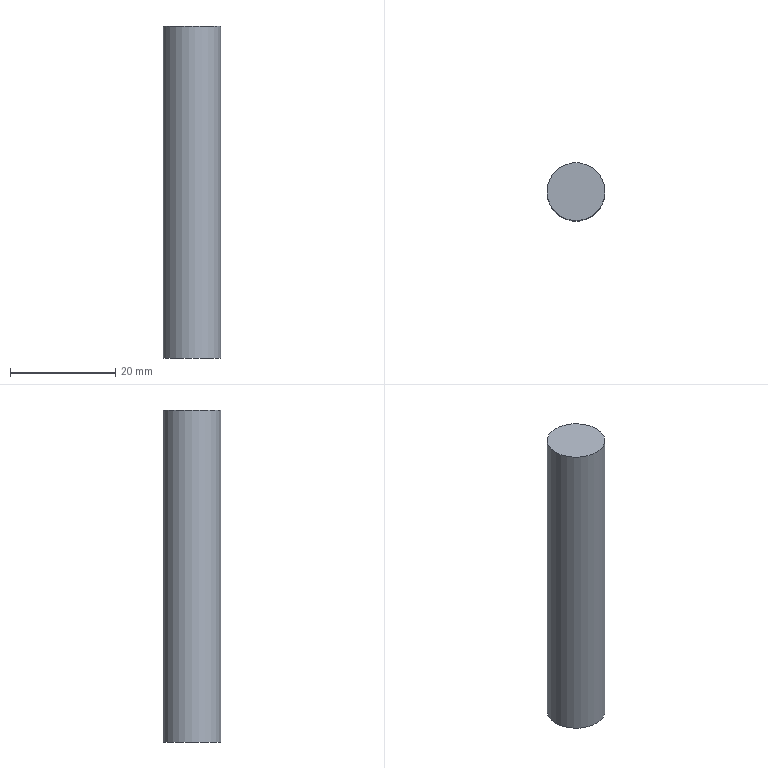Part | NX | features solid 2 | 1 solid | 3 faces | box 11 x 11 x 63 mm | volume 5987 mm3 | plane 2 | cylinder 1 | commonest cylinder face diameters 11 x1
STEP:
#1=CARTESIAN_POINT('',(117.465,-42.7,-79.4));
#2=VERTEX_POINT('',#1);
#3=CARTESIAN_POINT('',(111.965,-42.7,-79.4));
#4=DIRECTION('',(0.,0.,1.));
#5=DIRECTION('',(1.,0.,0.));
#6=AXIS2_PLACEMENT_3D('',#3,#4,#5);
#7=CIRCLE('',#6,5.5);
#8=EDGE_CURVE('',#2,#2,#7,.T.);
#9=ORIENTED_EDGE('',*,*,#8,.F.);
#10=EDGE_LOOP('',(#9));
#11=FACE_BOUND('',#10,.T.);
#12=CARTESIAN_POINT('',(117.465,-42.7,-142.4));
#13=VERTEX_POINT('',#12);
#14=CARTESIAN_POINT('',(111.965,-42.7,-142.4));
#15=DIRECTION('',(0.,0.,1.));
#16=DIRECTION('',(1.,0.,0.));
#17=AXIS2_PLACEMENT_3D('',#14,#15,#16);
#18=CIRCLE('',#17,5.5);
#19=EDGE_CURVE('',#13,#13,#18,.T.);
#20=ORIENTED_EDGE('',*,*,#19,.T.);
#21=EDGE_LOOP('',(#20));
#22=FACE_BOUND('',#21,.T.);
#23=CARTESIAN_POINT('',(111.965,-42.7,-79.4));
#24=DIRECTION('',(0.,0.,-1.));
#25=DIRECTION('',(-1.,0.,0.));
#26=AXIS2_PLACEMENT_3D('',#23,#24,#25);
#27=CYLINDRICAL_SURFACE('',#26,5.5);
#28=ADVANCED_FACE('',(#11,#22),#27,.T.);
#29=ORIENTED_EDGE('',*,*,#8,.T.);
#30=EDGE_LOOP('',(#29));
#31=FACE_BOUND('',#30,.T.);
#32=CARTESIAN_POINT('',(111.965,-42.7,-79.4));
#33=DIRECTION('',(0.,0.,1.));
#34=DIRECTION('',(1.,0.,0.));
#35=AXIS2_PLACEMENT_3D('',#32,#33,#34);
#36=PLANE('',#35);
#37=ADVANCED_FACE('',(#31),#36,.T.);
#38=ORIENTED_EDGE('',*,*,#19,.F.);
#39=EDGE_LOOP('',(#38));
#40=FACE_BOUND('',#39,.T.);
#41=CARTESIAN_POINT('',(111.965,-42.7,-142.4));
#42=DIRECTION('',(0.,0.,1.));
#43=DIRECTION('',(1.,0.,0.));
#44=AXIS2_PLACEMENT_3D('',#41,#42,#43);
#45=PLANE('',#44);
#46=ADVANCED_FACE('',(#40),#45,.F.);
#47=CLOSED_SHELL('',(#28,#37,#46));
#48=MANIFOLD_SOLID_BREP('',#47);
#49=(LENGTH_UNIT()NAMED_UNIT(*)SI_UNIT(.MILLI.,.METRE.));
#50=UNCERTAINTY_MEASURE_WITH_UNIT(LENGTH_MEASURE(0.00001),#49,'','');
#51=(NAMED_UNIT(*)PLANE_ANGLE_UNIT()SI_UNIT($,.RADIAN.));
#52=(NAMED_UNIT(*)SI_UNIT($,.STERADIAN.)SOLID_ANGLE_UNIT());
#53=(GEOMETRIC_REPRESENTATION_CONTEXT(3)GLOBAL_UNCERTAINTY_ASSIGNED_CONTEXT((#50))GLOBAL_UNIT_ASSIGNED_CONTEXT((#49,#51,#52))REPRESENTATION_CONTEXT('',''));
#54=ADVANCED_BREP_SHAPE_REPRESENTATION('',(#48),#53);